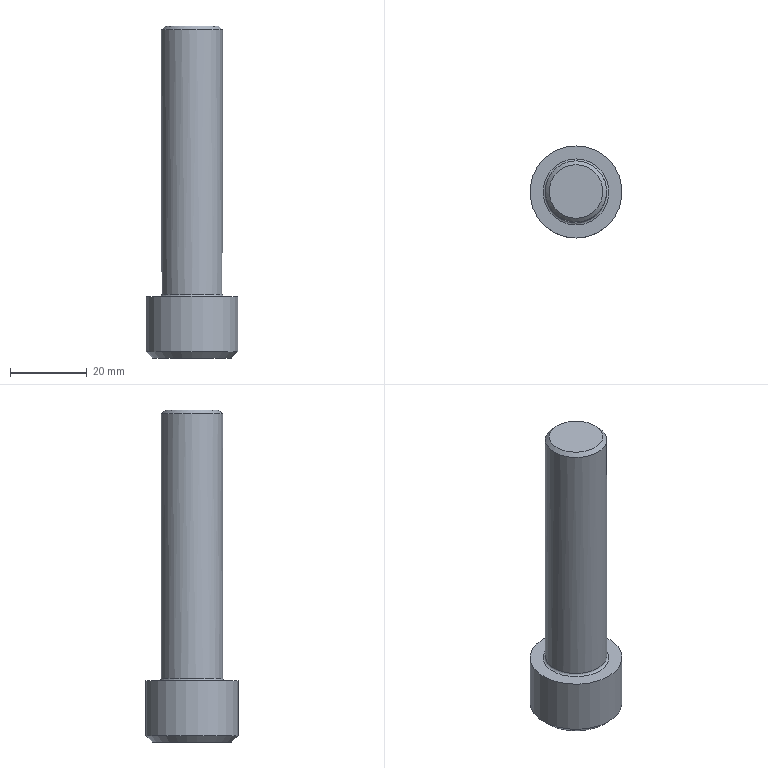Part | STEP file | solid 3 | 1 solid | 21 faces | box 24 x 24 x 86.5 mm | volume 19937 mm3 | plane 10 | sphere 6 | cylinder 2 | cone 2 | torus 1 | commonest cylinder face diameters 16 x1 24 x1